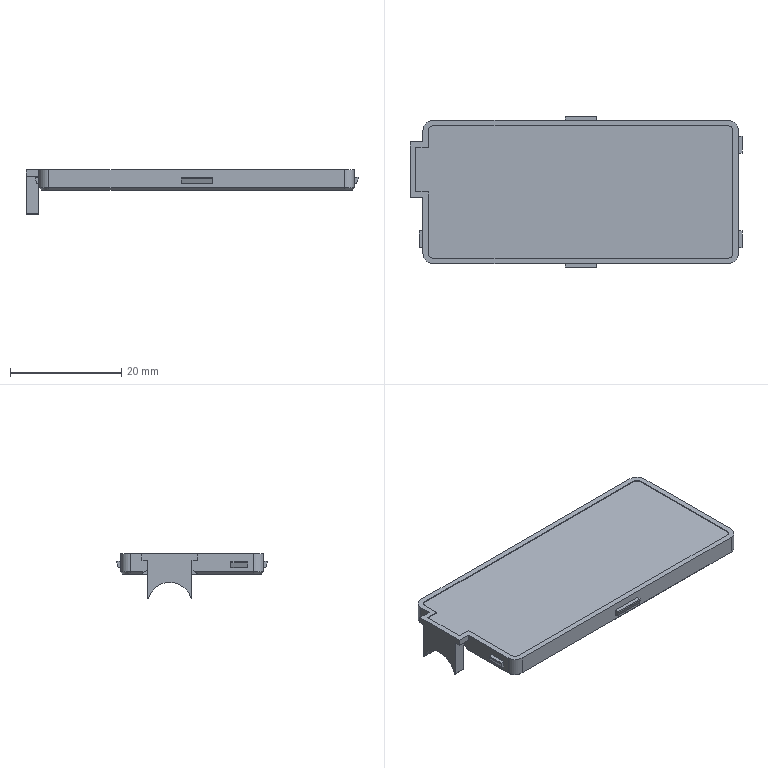Part | SolidWorks | features ICE 12, MirrorSolid 2, Chamfer 1, Cut 1, Extrusion 1, Fillet 1 | 4 solids | 106 faces | box 59.73 x 27.06 x 7.985 mm | volume 1980 mm3 | plane 70 | cylinder 28 | cone 4 | torus 4 | commonest cylinder face diameters 1.6 x8 0.5 x5 1 x5 3.6 x4 0.2 x2 8 x2